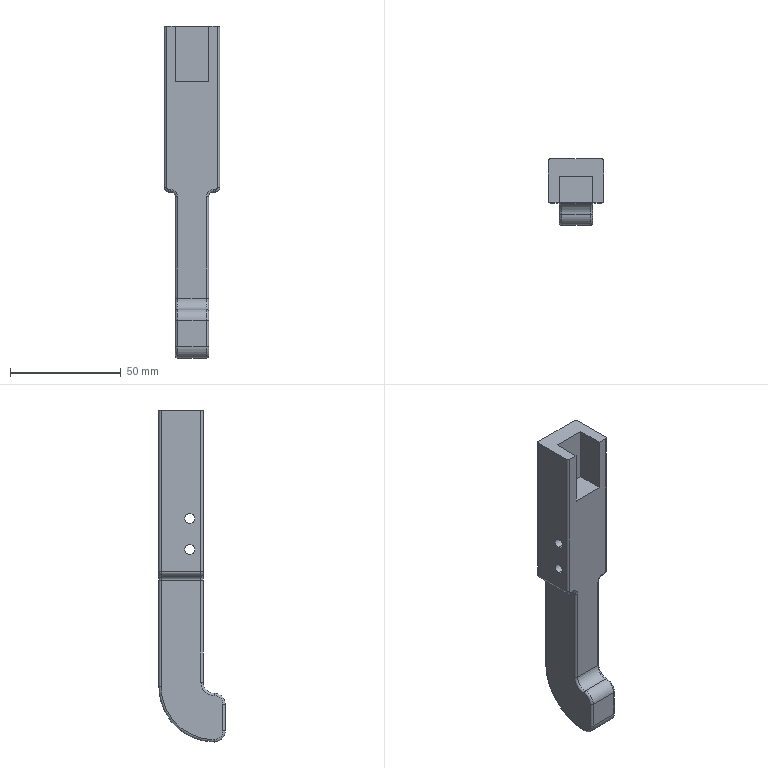Part | SolidWorks | features Fillet 5, ICE 3, Cut 1, Extrusion 1, HoleWzd 1 | 1 solid | 56 faces | box 25 x 30 x 150 mm | volume 55771 mm3 | cylinder 26 | torus 16 | plane 14 | commonest cylinder face diameters 2 x14 4 x4 4.5 x4 10 x3 50 x1